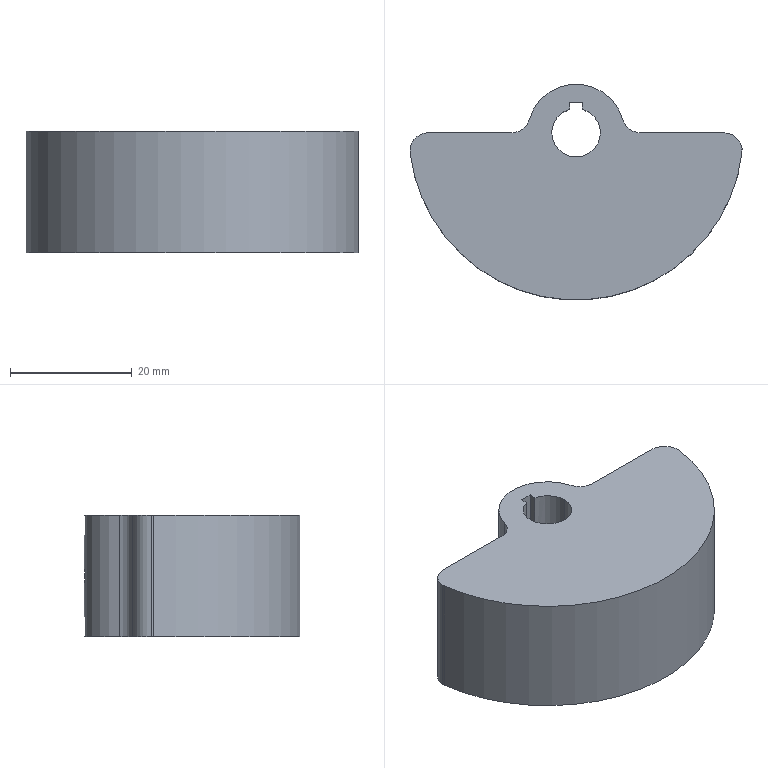Part | SolidWorks | features ICE 3, Extrusion 1, Fillet 1, HoleWzd 1 | 1 solid | 26 faces | box 54.631 x 35.5 x 20 mm | volume 24661 mm3 | cylinder 14 | plane 10 | cone 2 | commonest cylinder face diameters 6 x5 2.5 x4 8 x3 16 x1 55 x1
STEP:
#1=CARTESIAN_POINT('',(0.,-4.001,8.75));
#2=VERTEX_POINT('',#1);
#3=CARTESIAN_POINT('',(0.,-4.001,11.25));
#4=VERTEX_POINT('',#3);
#5=CARTESIAN_POINT('',(0.,-4.001,10.));
#6=DIRECTION('',(0.,1.,0.));
#7=DIRECTION('',(0.,0.,1.));
#8=AXIS2_PLACEMENT_3D('',#5,#6,#7);
#9=CIRCLE('',#8,1.25);
#10=EDGE_CURVE('',#2,#4,#9,.T.);
#11=ORIENTED_EDGE('',*,*,#10,.F.);
#12=CARTESIAN_POINT('',(0.,-4.,8.75));
#13=VERTEX_POINT('',#12);
#14=CARTESIAN_POINT('',(0.,8.,8.75));
#15=DIRECTION('',(0.,1.,0.));
#16=VECTOR('',#15,1000.);
#17=LINE('',#14,#16);
#18=EDGE_CURVE('',#2,#13,#17,.T.);
#19=ORIENTED_EDGE('',*,*,#18,.T.);
#20=CARTESIAN_POINT('',(0.,-4.,11.25));
#21=VERTEX_POINT('',#20);
#22=CARTESIAN_POINT('',(0.,-4.,11.25));
#23=CARTESIAN_POINT('',(-0.1663,-4.,11.25));
#24=CARTESIAN_POINT('',(-0.3294,-3.989,11.217));
#25=CARTESIAN_POINT('',(-0.6318,-3.953,11.091));
#26=CARTESIAN_POINT('',(-0.7697,-3.927,10.998));
#27=CARTESIAN_POINT('',(-0.9987,-3.875,10.769));
#28=CARTESIAN_POINT('',(-1.092,-3.849,10.63));
#29=CARTESIAN_POINT('',(-1.217,-3.811,10.33));
#30=CARTESIAN_POINT('',(-1.25,-3.8,10.165));
#31=CARTESIAN_POINT('',(-1.25,-3.8,9.918));
#32=CARTESIAN_POINT('',(-1.242,-3.802,9.835));
#33=CARTESIAN_POINT('',(-1.21,-3.813,9.674));
#34=CARTESIAN_POINT('',(-1.186,-3.82,9.596));
#35=CARTESIAN_POINT('',(-1.091,-3.849,9.368));
#36=CARTESIAN_POINT('',(-0.9989,-3.875,9.231));
#37=CARTESIAN_POINT('',(-0.8259,-3.914,9.058));
#38=CARTESIAN_POINT('',(-0.7634,-3.927,9.007));
#39=CARTESIAN_POINT('',(-0.6283,-3.951,8.916));
#40=CARTESIAN_POINT('',(-0.5551,-3.962,8.877));
#41=CARTESIAN_POINT('',(-0.3291,-3.989,8.783));
#42=CARTESIAN_POINT('',(-0.1639,-4.,8.75));
#43=CARTESIAN_POINT('',(0.,-4.,8.75));
#44=B_SPLINE_CURVE_WITH_KNOTS('',3,(#22,#23,#24,#25,#26,#27,#28,#29,#30,#31,#32,#33,#34,#35,#36,#37,#38,#39,#40,#41,#42,#43),.UNSPECIFIED.,.F.,.F.,(4,2,2,2,2,2,2,2,2,2,4),(0.,0.0004916,0.0009832,0.001475,0.001966,0.002212,0.002458,0.00295,0.003195,0.003441,0.003933),.UNSPECIFIED.);
#45=EDGE_CURVE('',#21,#13,#44,.T.);
#46=ORIENTED_EDGE('',*,*,#45,.F.);
#47=CARTESIAN_POINT('',(0.,8.,11.25));
#48=DIRECTION('',(0.,1.,0.));
#49=VECTOR('',#48,1000.);
#50=LINE('',#47,#49);
#51=EDGE_CURVE('',#4,#21,#50,.T.);
#52=ORIENTED_EDGE('',*,*,#51,.F.);
#53=EDGE_LOOP('',(#11,#19,#46,#52));
#54=FACE_OUTER_BOUND('',#53,.T.);
#55=CARTESIAN_POINT('',(0.,8.,10.));
#56=DIRECTION('',(0.,1.,0.));
#57=DIRECTION('',(0.,0.,1.));
#58=AXIS2_PLACEMENT_3D('',#55,#56,#57);
#59=CYLINDRICAL_SURFACE('',#58,1.25);
#60=ADVANCED_FACE('',(#54),#59,.F.);
#61=CARTESIAN_POINT('',(0.,-4.752,10.));
#62=VERTEX_POINT('',#61);
#63=CARTESIAN_POINT('',(0.,-4.001,11.25));
#64=DIRECTION('',(0.,0.515,0.8572));
#65=VECTOR('',#64,1000.);
#66=LINE('',#63,#65);
#67=EDGE_CURVE('',#62,#4,#66,.T.);
#68=ORIENTED_EDGE('',*,*,#67,.F.);
#69=CARTESIAN_POINT('',(0.,-4.001,8.75));
#70=DIRECTION('',(0.,0.515,-0.8572));
#71=VECTOR('',#70,1000.);
#72=LINE('',#69,#71);
#73=EDGE_CURVE('',#62,#2,#72,.T.);
#74=ORIENTED_EDGE('',*,*,#73,.T.);
#75=ORIENTED_EDGE('',*,*,#10,.T.);
#76=EDGE_LOOP('',(#68,#74,#75));
#77=FACE_OUTER_BOUND('',#76,.T.);
#78=CARTESIAN_POINT('',(0.,-4.001,10.));
#79=DIRECTION('',(0.,1.,0.));
#80=DIRECTION('',(0.,0.,1.));
#81=AXIS2_PLACEMENT_3D('',#78,#79,#80);
#82=CONICAL_SURFACE('',#81,1.25,1.03);
#83=ADVANCED_FACE('',(#77),#82,.F.);
#84=CARTESIAN_POINT('',(0.,5.,8.75));
#85=VERTEX_POINT('',#84);
#86=CARTESIAN_POINT('',(-1.,5.,9.25));
#87=VERTEX_POINT('',#86);
#88=CARTESIAN_POINT('',(0.,5.,10.));
#89=DIRECTION('',(0.,1.,0.));
#90=DIRECTION('',(0.,0.,1.));
#91=AXIS2_PLACEMENT_3D('',#88,#89,#90);
#92=CIRCLE('',#91,1.25);
#93=EDGE_CURVE('',#85,#87,#92,.T.);
#94=ORIENTED_EDGE('',*,*,#93,.F.);
#95=CARTESIAN_POINT('',(0.,8.,8.75));
#96=VERTEX_POINT('',#95);
#97=CARTESIAN_POINT('',(0.,8.,8.75));
#98=DIRECTION('',(0.,1.,0.));
#99=VECTOR('',#98,1000.);
#100=LINE('',#97,#99);
#101=EDGE_CURVE('',#85,#96,#100,.T.);
#102=ORIENTED_EDGE('',*,*,#101,.T.);
#103=CARTESIAN_POINT('',(0.,8.,11.25));
#104=VERTEX_POINT('',#103);
#105=CARTESIAN_POINT('',(0.,8.,8.75));
#106=CARTESIAN_POINT('',(-0.1633,8.,8.75));
#107=CARTESIAN_POINT('',(-0.3279,7.995,8.783));
#108=CARTESIAN_POINT('',(-0.6288,7.977,8.907));
#109=CARTESIAN_POINT('',(-0.768,7.964,9.));
#110=CARTESIAN_POINT('',(-0.941,7.945,9.173));
#111=CARTESIAN_POINT('',(-0.9937,7.938,9.237));
#112=CARTESIAN_POINT('',(-1.084,7.926,9.373));
#113=CARTESIAN_POINT('',(-1.123,7.921,9.445));
#114=CARTESIAN_POINT('',(-1.217,7.907,9.672));
#115=CARTESIAN_POINT('',(-1.25,7.902,9.834));
#116=CARTESIAN_POINT('',(-1.25,7.902,10.164));
#117=CARTESIAN_POINT('',(-1.218,7.907,10.327));
#118=CARTESIAN_POINT('',(-1.092,7.925,10.629));
#119=CARTESIAN_POINT('',(-0.9995,7.938,10.768));
#120=CARTESIAN_POINT('',(-0.7695,7.964,10.998));
#121=CARTESIAN_POINT('',(-0.6303,7.977,11.092));
#122=CARTESIAN_POINT('',(-0.3297,7.995,11.217));
#123=CARTESIAN_POINT('',(-0.1654,8.,11.25));
#124=CARTESIAN_POINT('',(0.,8.,11.25));
#125=B_SPLINE_CURVE_WITH_KNOTS('',3,(#105,#106,#107,#108,#109,#110,#111,#112,#113,#114,#115,#116,#117,#118,#119,#120,#121,#122,#123,#124),.UNSPECIFIED.,.F.,.F.,(4,2,2,2,2,2,2,2,2,4),(0.003914,0.004403,0.004892,0.005137,0.005381,0.005871,0.00636,0.006849,0.007338,0.007827),.UNSPECIFIED.);
#126=EDGE_CURVE('',#96,#104,#125,.T.);
#127=ORIENTED_EDGE('',*,*,#126,.T.);
#128=CARTESIAN_POINT('',(0.,5.,11.25));
#129=VERTEX_POINT('',#128);
#130=CARTESIAN_POINT('',(0.,8.,11.25));
#131=DIRECTION('',(0.,1.,0.));
#132=VECTOR('',#131,1000.);
#133=LINE('',#130,#132);
#134=EDGE_CURVE('',#129,#104,#133,.T.);
#135=ORIENTED_EDGE('',*,*,#134,.F.);
#136=CARTESIAN_POINT('',(-1.,5.,10.75));
#137=VERTEX_POINT('',#136);
#138=CARTESIAN_POINT('',(0.,5.,10.));
#139=DIRECTION('',(0.,1.,0.));
#140=DIRECTION('',(0.,0.,1.));
#141=AXIS2_PLACEMENT_3D('',#138,#139,#140);
#142=CIRCLE('',#141,1.25);
#143=EDGE_CURVE('',#137,#129,#142,.T.);
#144=ORIENTED_EDGE('',*,*,#143,.F.);
#145=CARTESIAN_POINT('',(-1.,3.873,10.75));
#146=VERTEX_POINT('',#145);
#147=CARTESIAN_POINT('',(-1.,8.,10.75));
#148=DIRECTION('',(0.,1.,0.));
#149=VECTOR('',#148,1000.);
#150=LINE('',#147,#149);
#151=EDGE_CURVE('',#146,#137,#150,.T.);
#152=ORIENTED_EDGE('',*,*,#151,.F.);
#153=CARTESIAN_POINT('',(-1.,3.873,9.25));
#154=VERTEX_POINT('',#153);
#155=CARTESIAN_POINT('',(-1.,3.873,9.25));
#156=CARTESIAN_POINT('',(-1.081,3.852,9.357));
#157=CARTESIAN_POINT('',(-1.142,3.834,9.475));
#158=CARTESIAN_POINT('',(-1.228,3.807,9.731));
#159=CARTESIAN_POINT('',(-1.25,3.8,9.864));
#160=CARTESIAN_POINT('',(-1.25,3.8,10.27));
#161=CARTESIAN_POINT('',(-1.161,3.831,10.535));
#162=CARTESIAN_POINT('',(-1.,3.873,10.75));
#163=B_SPLINE_CURVE_WITH_KNOTS('',3,(#155,#156,#157,#158,#159,#160,#161,#162),.UNSPECIFIED.,.F.,.F.,(4,2,2,4),(0.,0.0004023,0.0008046,0.001609),.UNSPECIFIED.);
#164=EDGE_CURVE('',#154,#146,#163,.T.);
#165=ORIENTED_EDGE('',*,*,#164,.F.);
#166=CARTESIAN_POINT('',(-1.,8.,9.25));
#167=DIRECTION('',(0.,-1.,0.));
#168=VECTOR('',#167,1000.);
#169=LINE('',#166,#168);
#170=EDGE_CURVE('',#87,#154,#169,.T.);
#171=ORIENTED_EDGE('',*,*,#170,.F.);
#172=EDGE_LOOP('',(#94,#102,#127,#135,#144,#152,#165,#171));
#173=FACE_OUTER_BOUND('',#172,.T.);
#174=CARTESIAN_POINT('',(0.,8.,10.));
#175=DIRECTION('',(0.,1.,0.));
#176=DIRECTION('',(0.,0.,1.));
#177=AXIS2_PLACEMENT_3D('',#174,#175,#176);
#178=CYLINDRICAL_SURFACE('',#177,1.25);
#179=ADVANCED_FACE('',(#173),#178,.F.);
#180=CARTESIAN_POINT('',(-27.316,-3.,20.));
#181=VERTEX_POINT('',#180);
#182=CARTESIAN_POINT('',(-27.293,-3.367,20.));
#183=VERTEX_POINT('',#182);
#184=CARTESIAN_POINT('',(-24.316,-3.,20.));
#185=DIRECTION('',(0.,0.,1.));
#186=DIRECTION('',(1.,0.,0.));
#187=AXIS2_PLACEMENT_3D('',#184,#185,#186);
#188=CIRCLE('',#187,3.);
#189=EDGE_CURVE('',#181,#183,#188,.T.);
#190=ORIENTED_EDGE('',*,*,#189,.F.);
#191=CARTESIAN_POINT('',(-27.316,-3.,0.));
#192=VERTEX_POINT('',#191);
#193=CARTESIAN_POINT('',(-27.316,-3.,20.));
#194=DIRECTION('',(0.,0.,-1.));
#195=VECTOR('',#194,1000.);
#196=LINE('',#193,#195);
#197=EDGE_CURVE('',#181,#192,#196,.T.);
#198=ORIENTED_EDGE('',*,*,#197,.T.);
#199=CARTESIAN_POINT('',(-27.293,-3.367,0.));
#200=VERTEX_POINT('',#199);
#201=CARTESIAN_POINT('',(-24.316,-3.,0.));
#202=DIRECTION('',(0.,0.,-1.));
#203=DIRECTION('',(1.,0.,0.));
#204=AXIS2_PLACEMENT_3D('',#201,#202,#203);
#205=CIRCLE('',#204,3.);
#206=EDGE_CURVE('',#200,#192,#205,.T.);
#207=ORIENTED_EDGE('',*,*,#206,.F.);
#208=CARTESIAN_POINT('',(-27.293,-3.367,20.));
#209=DIRECTION('',(0.,0.,-1.));
#210=VECTOR('',#209,1000.);
#211=LINE('',#208,#210);
#212=EDGE_CURVE('',#183,#200,#211,.T.);
#213=ORIENTED_EDGE('',*,*,#212,.F.);
#214=EDGE_LOOP('',(#190,#198,#207,#213));
#215=FACE_OUTER_BOUND('',#214,.T.);
#216=CARTESIAN_POINT('',(-24.316,-3.,20.));
#217=DIRECTION('',(0.,0.,-1.));
#218=DIRECTION('',(-1.,0.,0.));
#219=AXIS2_PLACEMENT_3D('',#216,#217,#218);
#220=CYLINDRICAL_SURFACE('',#219,3.);
#221=ADVANCED_FACE('',(#215),#220,.T.);
#222=ORIENTED_EDGE('',*,*,#45,.T.);
#223=CARTESIAN_POINT('',(0.,-4.,8.75));
#224=CARTESIAN_POINT('',(0.1638,-4.,8.75));
#225=CARTESIAN_POINT('',(0.3292,-3.989,8.783));
#226=CARTESIAN_POINT('',(0.6307,-3.953,8.908));
#227=CARTESIAN_POINT('',(0.7685,-3.927,9.001));
#228=CARTESIAN_POINT('',(0.9992,-3.875,9.231));
#229=CARTESIAN_POINT('',(1.091,-3.849,9.368));
#230=CARTESIAN_POINT('',(1.186,-3.82,9.596));
#231=CARTESIAN_POINT('',(1.21,-3.813,9.674));
#232=CARTESIAN_POINT('',(1.242,-3.802,9.834));
#233=CARTESIAN_POINT('',(1.25,-3.8,9.918));
#234=CARTESIAN_POINT('',(1.25,-3.8,10.165));
#235=CARTESIAN_POINT('',(1.217,-3.811,10.329));
#236=CARTESIAN_POINT('',(1.092,-3.849,10.631));
#237=CARTESIAN_POINT('',(0.9987,-3.875,10.769));
#238=CARTESIAN_POINT('',(0.7696,-3.927,10.998));
#239=CARTESIAN_POINT('',(0.6317,-3.953,11.091));
#240=CARTESIAN_POINT('',(0.3299,-3.989,11.217));
#241=CARTESIAN_POINT('',(0.1663,-4.,11.25));
#242=CARTESIAN_POINT('',(0.,-4.,11.25));
#243=B_SPLINE_CURVE_WITH_KNOTS('',3,(#223,#224,#225,#226,#227,#228,#229,#230,#231,#232,#233,#234,#235,#236,#237,#238,#239,#240,#241,#242),.UNSPECIFIED.,.F.,.F.,(4,2,2,2,2,2,2,2,2,4),(0.003933,0.004424,0.004916,0.005407,0.005653,0.005899,0.00639,0.006882,0.007373,0.007865),.UNSPECIFIED.);
#244=EDGE_CURVE('',#13,#21,#243,.T.);
#245=ORIENTED_EDGE('',*,*,#244,.T.);
#246=EDGE_LOOP('',(#222,#245));
#247=FACE_BOUND('',#246,.T.);
#248=CARTESIAN_POINT('',(-4.,0.,0.));
#249=VERTEX_POINT('',#248);
#250=CARTESIAN_POINT('',(4.,0.,0.));
#251=VERTEX_POINT('',#250);
#252=CARTESIAN_POINT('',(0.,0.,0.));
#253=DIRECTION('',(0.,0.,1.));
#254=DIRECTION('',(1.,0.,0.));
#255=AXIS2_PLACEMENT_3D('',#252,#253,#254);
#256=CIRCLE('',#255,4.);
#257=EDGE_CURVE('',#249,#251,#256,.T.);
#258=ORIENTED_EDGE('',*,*,#257,.F.);
#259=CARTESIAN_POINT('',(-4.,0.,20.));
#260=VERTEX_POINT('',#259);
#261=CARTESIAN_POINT('',(-4.,0.,0.));
#262=DIRECTION('',(0.,0.,1.));
#263=VECTOR('',#262,1000.);
#264=LINE('',#261,#263);
#265=EDGE_CURVE('',#249,#260,#264,.T.);
#266=ORIENTED_EDGE('',*,*,#265,.T.);
#267=CARTESIAN_POINT('',(4.,0.,20.));
#268=VERTEX_POINT('',#267);
#269=CARTESIAN_POINT('',(0.,0.,20.));
#270=DIRECTION('',(0.,0.,1.));
#271=DIRECTION('',(1.,0.,0.));
#272=AXIS2_PLACEMENT_3D('',#269,#270,#271);
#273=CIRCLE('',#272,4.);
#274=EDGE_CURVE('',#260,#268,#273,.T.);
#275=ORIENTED_EDGE('',*,*,#274,.T.);
#276=CARTESIAN_POINT('',(4.,0.,0.));
#277=DIRECTION('',(0.,0.,1.));
#278=VECTOR('',#277,1000.);
#279=LINE('',#276,#278);
#280=EDGE_CURVE('',#251,#268,#279,.T.);
#281=ORIENTED_EDGE('',*,*,#280,.F.);
#282=EDGE_LOOP('',(#258,#266,#275,#281));
#283=FACE_OUTER_BOUND('',#282,.T.);
#284=CARTESIAN_POINT('',(0.,0.,0.));
#285=DIRECTION('',(0.,0.,1.));
#286=DIRECTION('',(1.,0.,0.));
#287=AXIS2_PLACEMENT_3D('',#284,#285,#286);
#288=CYLINDRICAL_SURFACE('',#287,4.);
#289=ADVANCED_FACE('',(#247,#283),#288,.F.);
#290=CARTESIAN_POINT('',(1.,3.873,0.));
#291=VERTEX_POINT('',#290);
#292=CARTESIAN_POINT('',(0.,0.,0.));
#293=DIRECTION('',(0.,0.,1.));
#294=DIRECTION('',(1.,0.,0.));
#295=AXIS2_PLACEMENT_3D('',#292,#293,#294);
#296=CIRCLE('',#295,4.);
#297=EDGE_CURVE('',#251,#291,#296,.T.);
#298=ORIENTED_EDGE('',*,*,#297,.F.);
#299=ORIENTED_EDGE('',*,*,#280,.T.);
#300=CARTESIAN_POINT('',(1.,3.873,20.));
#301=VERTEX_POINT('',#300);
#302=CARTESIAN_POINT('',(0.,0.,20.));
#303=DIRECTION('',(0.,0.,1.));
#304=DIRECTION('',(1.,0.,0.));
#305=AXIS2_PLACEMENT_3D('',#302,#303,#304);
#306=CIRCLE('',#305,4.);
#307=EDGE_CURVE('',#268,#301,#306,.T.);
#308=ORIENTED_EDGE('',*,*,#307,.T.);
#309=CARTESIAN_POINT('',(1.,3.873,10.75));
#310=VERTEX_POINT('',#309);
#311=CARTESIAN_POINT('',(1.,3.873,0.));
#312=DIRECTION('',(0.,0.,-1.));
#313=VECTOR('',#312,1000.);
#314=LINE('',#311,#313);
#315=EDGE_CURVE('',#301,#310,#314,.T.);
#316=ORIENTED_EDGE('',*,*,#315,.T.);
#317=CARTESIAN_POINT('',(1.,3.873,9.25));
#318=VERTEX_POINT('',#317);
#319=CARTESIAN_POINT('',(1.,3.873,10.75));
#320=CARTESIAN_POINT('',(1.081,3.852,10.643));
#321=CARTESIAN_POINT('',(1.142,3.834,10.525));
#322=CARTESIAN_POINT('',(1.228,3.807,10.269));
#323=CARTESIAN_POINT('',(1.25,3.8,10.136));
#324=CARTESIAN_POINT('',(1.25,3.8,9.73));
#325=CARTESIAN_POINT('',(1.161,3.831,9.465));
#326=CARTESIAN_POINT('',(1.,3.873,9.25));
#327=B_SPLINE_CURVE_WITH_KNOTS('',3,(#319,#320,#321,#322,#323,#324,#325,#326),.UNSPECIFIED.,.F.,.F.,(4,2,2,4),(0.,0.0004023,0.0008046,0.001609),.UNSPECIFIED.);
#328=EDGE_CURVE('',#310,#318,#327,.T.);
#329=ORIENTED_EDGE('',*,*,#328,.T.);
#330=CARTESIAN_POINT('',(1.,3.873,0.));
#331=DIRECTION('',(0.,0.,-1.));
#332=VECTOR('',#331,1000.);
#333=LINE('',#330,#332);
#334=EDGE_CURVE('',#318,#291,#333,.T.);
#335=ORIENTED_EDGE('',*,*,#334,.T.);
#336=EDGE_LOOP('',(#298,#299,#308,#316,#329,#335));
#337=FACE_OUTER_BOUND('',#336,.T.);
#338=CARTESIAN_POINT('',(0.,0.,0.));
#339=DIRECTION('',(0.,0.,1.));
#340=DIRECTION('',(1.,0.,0.));
#341=AXIS2_PLACEMENT_3D('',#338,#339,#340);
#342=CYLINDRICAL_SURFACE('',#341,4.);
#343=ADVANCED_FACE('',(#337),#342,.F.);
#344=CARTESIAN_POINT('',(-1.,3.873,20.));
#345=VERTEX_POINT('',#344);
#346=CARTESIAN_POINT('',(-1.,3.873,0.));
#347=DIRECTION('',(0.,0.,1.));
#348=VECTOR('',#347,1000.);
#349=LINE('',#346,#348);
#350=EDGE_CURVE('',#146,#345,#349,.T.);
#351=ORIENTED_EDGE('',*,*,#350,.F.);
#352=ORIENTED_EDGE('',*,*,#151,.T.);
#353=CARTESIAN_POINT('',(-1.,5.,20.));
#354=VERTEX_POINT('',#353);
#355=CARTESIAN_POINT('',(-1.,5.,0.));
#356=DIRECTION('',(0.,0.,1.));
#357=VECTOR('',#356,1000.);
#358=LINE('',#355,#357);
#359=EDGE_CURVE('',#137,#354,#358,.T.);
#360=ORIENTED_EDGE('',*,*,#359,.T.);
#361=CARTESIAN_POINT('',(-1.,3.,20.));
#362=DIRECTION('',(0.,-1.,0.));
#363=VECTOR('',#362,1000.);
#364=LINE('',#361,#363);
#365=EDGE_CURVE('',#354,#345,#364,.T.);
#366=ORIENTED_EDGE('',*,*,#365,.T.);
#367=EDGE_LOOP('',(#351,#352,#360,#366));
#368=FACE_OUTER_BOUND('',#367,.T.);
#369=CARTESIAN_POINT('',(-1.,3.,0.));
#370=DIRECTION('',(-1.,0.,0.));
#371=DIRECTION('',(0.,0.,1.));
#372=AXIS2_PLACEMENT_3D('',#369,#370,#371);
#373=PLANE('',#372);
#374=ADVANCED_FACE('',(#368),#373,.F.);
#375=CARTESIAN_POINT('',(1.,5.,0.));
#376=VERTEX_POINT('',#375);
#377=CARTESIAN_POINT('',(1.,5.,9.25));
#378=VERTEX_POINT('',#377);
#379=CARTESIAN_POINT('',(1.,5.,0.));
#380=DIRECTION('',(0.,0.,1.));
#381=VECTOR('',#380,1000.);
#382=LINE('',#379,#381);
#383=EDGE_CURVE('',#376,#378,#382,.T.);
#384=ORIENTED_EDGE('',*,*,#383,.T.);
#385=CARTESIAN_POINT('',(0.,5.,10.));
#386=DIRECTION('',(0.,1.,0.));
#387=DIRECTION('',(0.,0.,1.));
#388=AXIS2_PLACEMENT_3D('',#385,#386,#387);
#389=CIRCLE('',#388,1.25);
#390=EDGE_CURVE('',#378,#85,#389,.T.);
#391=ORIENTED_EDGE('',*,*,#390,.T.);
#392=ORIENTED_EDGE('',*,*,#93,.T.);
#393=CARTESIAN_POINT('',(-1.,5.,0.));
#394=VERTEX_POINT('',#393);
#395=CARTESIAN_POINT('',(-1.,5.,0.));
#396=DIRECTION('',(0.,0.,1.));
#397=VECTOR('',#396,1000.);
#398=LINE('',#395,#397);
#399=EDGE_CURVE('',#394,#87,#398,.T.);
#400=ORIENTED_EDGE('',*,*,#399,.F.);
#401=CARTESIAN_POINT('',(-1.,5.,0.));
#402=DIRECTION('',(-1.,0.,0.));
#403=VECTOR('',#402,1000.);
#404=LINE('',#401,#403);
#405=EDGE_CURVE('',#376,#394,#404,.T.);
#406=ORIENTED_EDGE('',*,*,#405,.F.);
#407=EDGE_LOOP('',(#384,#391,#392,#400,#406));
#408=FACE_OUTER_BOUND('',#407,.T.);
#409=CARTESIAN_POINT('',(-1.,5.,0.));
#410=DIRECTION('',(0.,1.,0.));
#411=DIRECTION('',(0.,0.,1.));
#412=AXIS2_PLACEMENT_3D('',#409,#410,#411);
#413=PLANE('',#412);
#414=ADVANCED_FACE('',(#408),#413,.F.);
#415=ORIENTED_EDGE('',*,*,#334,.F.);
#416=CARTESIAN_POINT('',(1.,8.,9.25));
#417=DIRECTION('',(0.,1.,0.));
#418=VECTOR('',#417,1000.);
#419=LINE('',#416,#418);
#420=EDGE_CURVE('',#318,#378,#419,.T.);
#421=ORIENTED_EDGE('',*,*,#420,.T.);
#422=ORIENTED_EDGE('',*,*,#383,.F.);
#423=CARTESIAN_POINT('',(1.,3.,0.));
#424=DIRECTION('',(0.,1.,0.));
#425=VECTOR('',#424,1000.);
#426=LINE('',#423,#425);
#427=EDGE_CURVE('',#291,#376,#426,.T.);
#428=ORIENTED_EDGE('',*,*,#427,.F.);
#429=EDGE_LOOP('',(#415,#421,#422,#428));
#430=FACE_OUTER_BOUND('',#429,.T.);
#431=CARTESIAN_POINT('',(1.,3.,0.));
#432=DIRECTION('',(1.,0.,0.));
#433=DIRECTION('',(0.,0.,-1.));
#434=AXIS2_PLACEMENT_3D('',#431,#432,#433);
#435=PLANE('',#434);
#436=ADVANCED_FACE('',(#430),#435,.F.);
#437=CARTESIAN_POINT('',(24.316,0.,20.));
#438=VERTEX_POINT('',#437);
#439=CARTESIAN_POINT('',(10.583,0.,20.));
#440=VERTEX_POINT('',#439);
#441=CARTESIAN_POINT('',(-27.5,0.,20.));
#442=DIRECTION('',(-1.,0.,0.));
#443=VECTOR('',#442,1000.);
#444=LINE('',#441,#443);
#445=EDGE_CURVE('',#438,#440,#444,.T.);
#446=ORIENTED_EDGE('',*,*,#445,.F.);
#447=CARTESIAN_POINT('',(24.316,0.,0.));
#448=VERTEX_POINT('',#447);
#449=CARTESIAN_POINT('',(24.316,0.,20.));
#450=DIRECTION('',(0.,0.,-1.));
#451=VECTOR('',#450,1000.);
#452=LINE('',#449,#451);
#453=EDGE_CURVE('',#438,#448,#452,.T.);
#454=ORIENTED_EDGE('',*,*,#453,.T.);
#455=CARTESIAN_POINT('',(10.583,0.,0.));
#456=VERTEX_POINT('',#455);
#457=CARTESIAN_POINT('',(-27.5,0.,0.));
#458=DIRECTION('',(-1.,0.,0.));
#459=VECTOR('',#458,1000.);
#460=LINE('',#457,#459);
#461=EDGE_CURVE('',#448,#456,#460,.T.);
#462=ORIENTED_EDGE('',*,*,#461,.T.);
#463=CARTESIAN_POINT('',(10.583,0.,20.));
#464=DIRECTION('',(0.,0.,1.));
#465=VECTOR('',#464,1000.);
#466=LINE('',#463,#465);
#467=EDGE_CURVE('',#456,#440,#466,.T.);
#468=ORIENTED_EDGE('',*,*,#467,.T.);
#469=EDGE_LOOP('',(#446,#454,#462,#468));
#470=FACE_OUTER_BOUND('',#469,.T.);
#471=CARTESIAN_POINT('',(-27.5,0.,20.));
#472=DIRECTION('',(0.,-1.,0.));
#473=DIRECTION('',(0.,0.,-1.));
#474=AXIS2_PLACEMENT_3D('',#471,#472,#473);
#475=PLANE('',#474);
#476=ADVANCED_FACE('',(#470),#475,.F.);
#477=CARTESIAN_POINT('',(27.293,-3.367,0.));
#478=VERTEX_POINT('',#477);
#479=CARTESIAN_POINT('',(0.,0.,0.));
#480=DIRECTION('',(0.,0.,1.));
#481=DIRECTION('',(1.,0.,0.));
#482=AXIS2_PLACEMENT_3D('',#479,#480,#481);
#483=CIRCLE('',#482,27.5);
#484=EDGE_CURVE('',#200,#478,#483,.T.);
#485=ORIENTED_EDGE('',*,*,#484,.T.);
#486=CARTESIAN_POINT('',(27.293,-3.367,20.));
#487=VERTEX_POINT('',#486);
#488=CARTESIAN_POINT('',(27.293,-3.367,20.));
#489=DIRECTION('',(0.,0.,1.));
#490=VECTOR('',#489,1000.);
#491=LINE('',#488,#490);
#492=EDGE_CURVE('',#478,#487,#491,.T.);
#493=ORIENTED_EDGE('',*,*,#492,.T.);
#494=CARTESIAN_POINT('',(0.,0.,20.));
#495=DIRECTION('',(0.,0.,1.));
#496=DIRECTION('',(1.,0.,0.));
#497=AXIS2_PLACEMENT_3D('',#494,#495,#496);
#498=CIRCLE('',#497,27.5);
#499=EDGE_CURVE('',#183,#487,#498,.T.);
#500=ORIENTED_EDGE('',*,*,#499,.F.);
#501=ORIENTED_EDGE('',*,*,#212,.T.);
#502=EDGE_LOOP('',(#485,#493,#500,#501));
#503=FACE_OUTER_BOUND('',#502,.T.);
#504=CARTESIAN_POINT('',(0.,0.,20.));
#505=DIRECTION('',(0.,0.,-1.));
#506=DIRECTION('',(-1.,0.,0.));
#507=AXIS2_PLACEMENT_3D('',#504,#505,#506);
#508=CYLINDRICAL_SURFACE('',#507,27.5);
#509=ADVANCED_FACE('',(#503),#508,.T.);
#510=CARTESIAN_POINT('',(-10.583,0.,20.));
#511=VERTEX_POINT('',#510);
#512=CARTESIAN_POINT('',(-24.316,0.,20.));
#513=VERTEX_POINT('',#512);
#514=CARTESIAN_POINT('',(-27.5,0.,20.));
#515=DIRECTION('',(-1.,0.,0.));
#516=VECTOR('',#515,1000.);
#517=LINE('',#514,#516);
#518=EDGE_CURVE('',#511,#513,#517,.T.);
#519=ORIENTED_EDGE('',*,*,#518,.F.);
#520=CARTESIAN_POINT('',(-10.583,0.,0.));
#521=VERTEX_POINT('',#520);
#522=CARTESIAN_POINT('',(-10.583,0.,20.));
#523=DIRECTION('',(0.,0.,-1.));
#524=VECTOR('',#523,1000.);
#525=LINE('',#522,#524);
#526=EDGE_CURVE('',#511,#521,#525,.T.);
#527=ORIENTED_EDGE('',*,*,#526,.T.);
#528=CARTESIAN_POINT('',(-24.316,0.,0.));
#529=VERTEX_POINT('',#528);
#530=CARTESIAN_POINT('',(-27.5,0.,0.));
#531=DIRECTION('',(-1.,0.,0.));
#532=VECTOR('',#531,1000.);
#533=LINE('',#530,#532);
#534=EDGE_CURVE('',#521,#529,#533,.T.);
#535=ORIENTED_EDGE('',*,*,#534,.T.);
#536=CARTESIAN_POINT('',(-24.316,0.,20.));
#537=DIRECTION('',(0.,0.,1.));
#538=VECTOR('',#537,1000.);
#539=LINE('',#536,#538);
#540=EDGE_CURVE('',#529,#513,#539,.T.);
#541=ORIENTED_EDGE('',*,*,#540,.T.);
#542=EDGE_LOOP('',(#519,#527,#535,#541));
#543=FACE_OUTER_BOUND('',#542,.T.);
#544=CARTESIAN_POINT('',(-27.5,0.,20.));
#545=DIRECTION('',(0.,-1.,0.));
#546=DIRECTION('',(0.,0.,-1.));
#547=AXIS2_PLACEMENT_3D('',#544,#545,#546);
#548=PLANE('',#547);
#549=ADVANCED_FACE('',(#543),#548,.F.);
#550=CARTESIAN_POINT('',(1.,5.,20.));
#551=VERTEX_POINT('',#550);
#552=CARTESIAN_POINT('',(1.,3.,20.));
#553=DIRECTION('',(0.,1.,0.));
#554=VECTOR('',#553,1000.);
#555=LINE('',#552,#554);
#556=EDGE_CURVE('',#301,#551,#555,.T.);
#557=ORIENTED_EDGE('',*,*,#556,.F.);
#558=ORIENTED_EDGE('',*,*,#307,.F.);
#559=ORIENTED_EDGE('',*,*,#274,.F.);
#560=CARTESIAN_POINT('',(0.,0.,20.));
#561=DIRECTION('',(0.,0.,1.));
#562=DIRECTION('',(1.,0.,0.));
#563=AXIS2_PLACEMENT_3D('',#560,#561,#562);
#564=CIRCLE('',#563,4.);
#565=EDGE_CURVE('',#345,#260,#564,.T.);
#566=ORIENTED_EDGE('',*,*,#565,.F.);
#567=ORIENTED_EDGE('',*,*,#365,.F.);
#568=CARTESIAN_POINT('',(-1.,5.,20.));
#569=DIRECTION('',(-1.,0.,0.));
#570=VECTOR('',#569,1000.);
#571=LINE('',#568,#570);
#572=EDGE_CURVE('',#551,#354,#571,.T.);
#573=ORIENTED_EDGE('',*,*,#572,.F.);
#574=EDGE_LOOP('',(#557,#558,#559,#566,#567,#573));
#575=FACE_BOUND('',#574,.T.);
#576=ORIENTED_EDGE('',*,*,#499,.T.);
#577=CARTESIAN_POINT('',(24.316,-3.,20.));
#578=DIRECTION('',(0.,0.,1.));
#579=DIRECTION('',(1.,0.,0.));
#580=AXIS2_PLACEMENT_3D('',#577,#578,#579);
#581=CIRCLE('',#580,3.);
#582=EDGE_CURVE('',#487,#438,#581,.T.);
#583=ORIENTED_EDGE('',*,*,#582,.T.);
#584=ORIENTED_EDGE('',*,*,#445,.T.);
#585=CARTESIAN_POINT('',(7.697,2.182,20.));
#586=VERTEX_POINT('',#585);
#587=CARTESIAN_POINT('',(10.583,3.,20.));
#588=DIRECTION('',(0.,0.,-1.));
#589=DIRECTION('',(1.,0.,0.));
#590=AXIS2_PLACEMENT_3D('',#587,#588,#589);
#591=CIRCLE('',#590,3.);
#592=EDGE_CURVE('',#440,#586,#591,.T.);
#593=ORIENTED_EDGE('',*,*,#592,.T.);
#594=CARTESIAN_POINT('',(-7.697,2.182,20.));
#595=VERTEX_POINT('',#594);
#596=CARTESIAN_POINT('',(0.,0.,20.));
#597=DIRECTION('',(0.,0.,1.));
#598=DIRECTION('',(1.,0.,0.));
#599=AXIS2_PLACEMENT_3D('',#596,#597,#598);
#600=CIRCLE('',#599,8.);
#601=EDGE_CURVE('',#586,#595,#600,.T.);
#602=ORIENTED_EDGE('',*,*,#601,.T.);
#603=CARTESIAN_POINT('',(-10.583,3.,20.));
#604=DIRECTION('',(0.,0.,-1.));
#605=DIRECTION('',(1.,0.,0.));
#606=AXIS2_PLACEMENT_3D('',#603,#604,#605);
#607=CIRCLE('',#606,3.);
#608=EDGE_CURVE('',#595,#511,#607,.T.);
#609=ORIENTED_EDGE('',*,*,#608,.T.);
#610=ORIENTED_EDGE('',*,*,#518,.T.);
#611=CARTESIAN_POINT('',(-24.316,-3.,20.));
#612=DIRECTION('',(0.,0.,1.));
#613=DIRECTION('',(1.,0.,0.));
#614=AXIS2_PLACEMENT_3D('',#611,#612,#613);
#615=CIRCLE('',#614,3.);
#616=EDGE_CURVE('',#513,#181,#615,.T.);
#617=ORIENTED_EDGE('',*,*,#616,.T.);
#618=ORIENTED_EDGE('',*,*,#189,.T.);
#619=EDGE_LOOP('',(#576,#583,#584,#593,#602,#609,#610,#617,#618));
#620=FACE_OUTER_BOUND('',#619,.T.);
#621=CARTESIAN_POINT('',(0.,0.,20.));
#622=DIRECTION('',(0.,0.,1.));
#623=DIRECTION('',(1.,0.,0.));
#624=AXIS2_PLACEMENT_3D('',#621,#622,#623);
#625=PLANE('',#624);
#626=ADVANCED_FACE('',(#575,#620),#625,.T.);
#627=CARTESIAN_POINT('',(-1.,3.873,0.));
#628=VERTEX_POINT('',#627);
#629=CARTESIAN_POINT('',(0.,0.,0.));
#630=DIRECTION('',(0.,0.,1.));
#631=DIRECTION('',(1.,0.,0.));
#632=AXIS2_PLACEMENT_3D('',#629,#630,#631);
#633=CIRCLE('',#632,4.);
#634=EDGE_CURVE('',#628,#249,#633,.T.);
#635=ORIENTED_EDGE('',*,*,#634,.T.);
#636=ORIENTED_EDGE('',*,*,#257,.T.);
#637=ORIENTED_EDGE('',*,*,#297,.T.);
#638=ORIENTED_EDGE('',*,*,#427,.T.);
#639=ORIENTED_EDGE('',*,*,#405,.T.);
#640=CARTESIAN_POINT('',(-1.,3.,0.));
#641=DIRECTION('',(0.,-1.,0.));
#642=VECTOR('',#641,1000.);
#643=LINE('',#640,#642);
#644=EDGE_CURVE('',#394,#628,#643,.T.);
#645=ORIENTED_EDGE('',*,*,#644,.T.);
#646=EDGE_LOOP('',(#635,#636,#637,#638,#639,#645));
#647=FACE_BOUND('',#646,.T.);
#648=ORIENTED_EDGE('',*,*,#461,.F.);
#649=CARTESIAN_POINT('',(24.316,-3.,0.));
#650=DIRECTION('',(0.,0.,-1.));
#651=DIRECTION('',(1.,0.,0.));
#652=AXIS2_PLACEMENT_3D('',#649,#650,#651);
#653=CIRCLE('',#652,3.);
#654=EDGE_CURVE('',#448,#478,#653,.T.);
#655=ORIENTED_EDGE('',*,*,#654,.T.);
#656=ORIENTED_EDGE('',*,*,#484,.F.);
#657=ORIENTED_EDGE('',*,*,#206,.T.);
#658=CARTESIAN_POINT('',(-24.316,-3.,0.));
#659=DIRECTION('',(0.,0.,-1.));
#660=DIRECTION('',(1.,0.,0.));
#661=AXIS2_PLACEMENT_3D('',#658,#659,#660);
#662=CIRCLE('',#661,3.);
#663=EDGE_CURVE('',#192,#529,#662,.T.);
#664=ORIENTED_EDGE('',*,*,#663,.T.);
#665=ORIENTED_EDGE('',*,*,#534,.F.);
#666=CARTESIAN_POINT('',(-7.697,2.182,0.));
#667=VERTEX_POINT('',#666);
#668=CARTESIAN_POINT('',(-10.583,3.,0.));
#669=DIRECTION('',(0.,0.,1.));
#670=DIRECTION('',(1.,0.,0.));
#671=AXIS2_PLACEMENT_3D('',#668,#669,#670);
#672=CIRCLE('',#671,3.);
#673=EDGE_CURVE('',#521,#667,#672,.T.);
#674=ORIENTED_EDGE('',*,*,#673,.T.);
#675=CARTESIAN_POINT('',(7.697,2.182,0.));
#676=VERTEX_POINT('',#675);
#677=CARTESIAN_POINT('',(0.,0.,0.));
#678=DIRECTION('',(0.,0.,1.));
#679=DIRECTION('',(1.,0.,0.));
#680=AXIS2_PLACEMENT_3D('',#677,#678,#679);
#681=CIRCLE('',#680,8.);
#682=EDGE_CURVE('',#676,#667,#681,.T.);
#683=ORIENTED_EDGE('',*,*,#682,.F.);
#684=CARTESIAN_POINT('',(10.583,3.,0.));
#685=DIRECTION('',(0.,0.,1.));
#686=DIRECTION('',(1.,0.,0.));
#687=AXIS2_PLACEMENT_3D('',#684,#685,#686);
#688=CIRCLE('',#687,3.);
#689=EDGE_CURVE('',#676,#456,#688,.T.);
#690=ORIENTED_EDGE('',*,*,#689,.T.);
#691=EDGE_LOOP('',(#648,#655,#656,#657,#664,#665,#674,#683,#690));
#692=FACE_OUTER_BOUND('',#691,.T.);
#693=CARTESIAN_POINT('',(0.,0.,0.));
#694=DIRECTION('',(0.,0.,1.));
#695=DIRECTION('',(1.,0.,0.));
#696=AXIS2_PLACEMENT_3D('',#693,#694,#695);
#697=PLANE('',#696);
#698=ADVANCED_FACE('',(#647,#692),#697,.F.);
#699=CARTESIAN_POINT('',(0.,8.,11.25));
#700=CARTESIAN_POINT('',(0.1655,8.,11.25));
#701=CARTESIAN_POINT('',(0.3278,7.995,11.217));
#702=CARTESIAN_POINT('',(0.6305,7.977,11.092));
#703=CARTESIAN_POINT('',(0.769,7.964,10.999));
#704=CARTESIAN_POINT('',(0.9992,7.938,10.769));
#705=CARTESIAN_POINT('',(1.092,7.925,10.629));
#706=CARTESIAN_POINT('',(1.217,7.907,10.328));
#707=CARTESIAN_POINT('',(1.25,7.902,10.164));
#708=CARTESIAN_POINT('',(1.25,7.902,9.919));
#709=CARTESIAN_POINT('',(1.242,7.903,9.836));
#710=CARTESIAN_POINT('',(1.21,7.908,9.675));
#711=CARTESIAN_POINT('',(1.186,7.912,9.597));
#712=CARTESIAN_POINT('',(1.092,7.925,9.37));
#713=CARTESIAN_POINT('',(1.,7.938,9.233));
#714=CARTESIAN_POINT('',(0.7675,7.964,9.));
#715=CARTESIAN_POINT('',(0.6299,7.977,8.908));
#716=CARTESIAN_POINT('',(0.403,7.99,8.814));
#717=CARTESIAN_POINT('',(0.3251,7.994,8.79));
#718=CARTESIAN_POINT('',(0.1646,7.999,8.758));
#719=CARTESIAN_POINT('',(0.08165,8.,8.75));
#720=CARTESIAN_POINT('',(0.,8.,8.75));
#721=B_SPLINE_CURVE_WITH_KNOTS('',3,(#699,#700,#701,#702,#703,#704,#705,#706,#707,#708,#709,#710,#711,#712,#713,#714,#715,#716,#717,#718,#719,#720),.UNSPECIFIED.,.F.,.F.,(4,2,2,2,2,2,2,2,2,2,4),(0.,0.0004893,0.0009785,0.001468,0.001957,0.002202,0.002446,0.002936,0.003425,0.003669,0.003914),.UNSPECIFIED.);
#722=EDGE_CURVE('',#104,#96,#721,.T.);
#723=ORIENTED_EDGE('',*,*,#722,.F.);
#724=ORIENTED_EDGE('',*,*,#126,.F.);
#725=EDGE_LOOP('',(#723,#724));
#726=FACE_BOUND('',#725,.T.);
#727=ORIENTED_EDGE('',*,*,#601,.F.);
#728=CARTESIAN_POINT('',(7.697,2.182,0.));
#729=DIRECTION('',(0.,0.,-1.));
#730=VECTOR('',#729,1000.);
#731=LINE('',#728,#730);
#732=EDGE_CURVE('',#586,#676,#731,.T.);
#733=ORIENTED_EDGE('',*,*,#732,.T.);
#734=ORIENTED_EDGE('',*,*,#682,.T.);
#735=CARTESIAN_POINT('',(-7.697,2.182,0.));
#736=DIRECTION('',(0.,0.,1.));
#737=VECTOR('',#736,1000.);
#738=LINE('',#735,#737);
#739=EDGE_CURVE('',#667,#595,#738,.T.);
#740=ORIENTED_EDGE('',*,*,#739,.T.);
#741=EDGE_LOOP('',(#727,#733,#734,#740));
#742=FACE_OUTER_BOUND('',#741,.T.);
#743=CARTESIAN_POINT('',(0.,0.,0.));
#744=DIRECTION('',(0.,0.,1.));
#745=DIRECTION('',(1.,0.,0.));
#746=AXIS2_PLACEMENT_3D('',#743,#744,#745);
#747=CYLINDRICAL_SURFACE('',#746,8.);
#748=ADVANCED_FACE('',(#726,#742),#747,.T.);
#749=ORIENTED_EDGE('',*,*,#265,.F.);
#750=ORIENTED_EDGE('',*,*,#634,.F.);
#751=CARTESIAN_POINT('',(-1.,3.873,0.));
#752=DIRECTION('',(0.,0.,1.));
#753=VECTOR('',#752,1000.);
#754=LINE('',#751,#753);
#755=EDGE_CURVE('',#628,#154,#754,.T.);
#756=ORIENTED_EDGE('',*,*,#755,.T.);
#757=ORIENTED_EDGE('',*,*,#164,.T.);
#758=ORIENTED_EDGE('',*,*,#350,.T.);
#759=ORIENTED_EDGE('',*,*,#565,.T.);
#760=EDGE_LOOP('',(#749,#750,#756,#757,#758,#759));
#761=FACE_OUTER_BOUND('',#760,.T.);
#762=CARTESIAN_POINT('',(0.,0.,0.));
#763=DIRECTION('',(0.,0.,1.));
#764=DIRECTION('',(1.,0.,0.));
#765=AXIS2_PLACEMENT_3D('',#762,#763,#764);
#766=CYLINDRICAL_SURFACE('',#765,4.);
#767=ADVANCED_FACE('',(#761),#766,.F.);
#768=ORIENTED_EDGE('',*,*,#582,.F.);
#769=ORIENTED_EDGE('',*,*,#492,.F.);
#770=ORIENTED_EDGE('',*,*,#654,.F.);
#771=ORIENTED_EDGE('',*,*,#453,.F.);
#772=EDGE_LOOP('',(#768,#769,#770,#771));
#773=FACE_OUTER_BOUND('',#772,.T.);
#774=CARTESIAN_POINT('',(24.316,-3.,20.));
#775=DIRECTION('',(0.,0.,-1.));
#776=DIRECTION('',(-1.,0.,0.));
#777=AXIS2_PLACEMENT_3D('',#774,#775,#776);
#778=CYLINDRICAL_SURFACE('',#777,3.);
#779=ADVANCED_FACE('',(#773),#778,.T.);
#780=ORIENTED_EDGE('',*,*,#689,.F.);
#781=ORIENTED_EDGE('',*,*,#732,.F.);
#782=ORIENTED_EDGE('',*,*,#592,.F.);
#783=ORIENTED_EDGE('',*,*,#467,.F.);
#784=EDGE_LOOP('',(#780,#781,#782,#783));
#785=FACE_OUTER_BOUND('',#784,.T.);
#786=CARTESIAN_POINT('',(10.583,3.,0.));
#787=DIRECTION('',(0.,0.,1.));
#788=DIRECTION('',(1.,0.,0.));
#789=AXIS2_PLACEMENT_3D('',#786,#787,#788);
#790=CYLINDRICAL_SURFACE('',#789,3.);
#791=ADVANCED_FACE('',(#785),#790,.F.);
#792=ORIENTED_EDGE('',*,*,#608,.F.);
#793=ORIENTED_EDGE('',*,*,#739,.F.);
#794=ORIENTED_EDGE('',*,*,#673,.F.);
#795=ORIENTED_EDGE('',*,*,#526,.F.);
#796=EDGE_LOOP('',(#792,#793,#794,#795));
#797=FACE_OUTER_BOUND('',#796,.T.);
#798=CARTESIAN_POINT('',(-10.583,3.,0.));
#799=DIRECTION('',(0.,0.,1.));
#800=DIRECTION('',(1.,0.,0.));
#801=AXIS2_PLACEMENT_3D('',#798,#799,#800);
#802=CYLINDRICAL_SURFACE('',#801,3.);
#803=ADVANCED_FACE('',(#797),#802,.F.);
#804=ORIENTED_EDGE('',*,*,#197,.F.);
#805=ORIENTED_EDGE('',*,*,#616,.F.);
#806=ORIENTED_EDGE('',*,*,#540,.F.);
#807=ORIENTED_EDGE('',*,*,#663,.F.);
#808=EDGE_LOOP('',(#804,#805,#806,#807));
#809=FACE_OUTER_BOUND('',#808,.T.);
#810=CARTESIAN_POINT('',(-24.316,-3.,20.));
#811=DIRECTION('',(0.,0.,-1.));
#812=DIRECTION('',(-1.,0.,0.));
#813=AXIS2_PLACEMENT_3D('',#810,#811,#812);
#814=CYLINDRICAL_SURFACE('',#813,3.);
#815=ADVANCED_FACE('',(#809),#814,.T.);
#816=CARTESIAN_POINT('',(1.,5.,10.75));
#817=VERTEX_POINT('',#816);
#818=CARTESIAN_POINT('',(1.,5.,0.));
#819=DIRECTION('',(0.,0.,1.));
#820=VECTOR('',#819,1000.);
#821=LINE('',#818,#820);
#822=EDGE_CURVE('',#817,#551,#821,.T.);
#823=ORIENTED_EDGE('',*,*,#822,.F.);
#824=CARTESIAN_POINT('',(1.,8.,10.75));
#825=DIRECTION('',(0.,-1.,0.));
#826=VECTOR('',#825,1000.);
#827=LINE('',#824,#826);
#828=EDGE_CURVE('',#817,#310,#827,.T.);
#829=ORIENTED_EDGE('',*,*,#828,.T.);
#830=ORIENTED_EDGE('',*,*,#315,.F.);
#831=ORIENTED_EDGE('',*,*,#556,.T.);
#832=EDGE_LOOP('',(#823,#829,#830,#831));
#833=FACE_OUTER_BOUND('',#832,.T.);
#834=CARTESIAN_POINT('',(1.,3.,0.));
#835=DIRECTION('',(1.,0.,0.));
#836=DIRECTION('',(0.,0.,-1.));
#837=AXIS2_PLACEMENT_3D('',#834,#835,#836);
#838=PLANE('',#837);
#839=ADVANCED_FACE('',(#833),#838,.F.);
#840=ORIENTED_EDGE('',*,*,#399,.T.);
#841=ORIENTED_EDGE('',*,*,#170,.T.);
#842=ORIENTED_EDGE('',*,*,#755,.F.);
#843=ORIENTED_EDGE('',*,*,#644,.F.);
#844=EDGE_LOOP('',(#840,#841,#842,#843));
#845=FACE_OUTER_BOUND('',#844,.T.);
#846=CARTESIAN_POINT('',(-1.,3.,0.));
#847=DIRECTION('',(-1.,0.,0.));
#848=DIRECTION('',(0.,0.,1.));
#849=AXIS2_PLACEMENT_3D('',#846,#847,#848);
#850=PLANE('',#849);
#851=ADVANCED_FACE('',(#845),#850,.F.);
#852=ORIENTED_EDGE('',*,*,#359,.F.);
#853=ORIENTED_EDGE('',*,*,#143,.T.);
#854=CARTESIAN_POINT('',(0.,5.,10.));
#855=DIRECTION('',(0.,1.,0.));
#856=DIRECTION('',(0.,0.,1.));
#857=AXIS2_PLACEMENT_3D('',#854,#855,#856);
#858=CIRCLE('',#857,1.25);
#859=EDGE_CURVE('',#129,#817,#858,.T.);
#860=ORIENTED_EDGE('',*,*,#859,.T.);
#861=ORIENTED_EDGE('',*,*,#822,.T.);
#862=ORIENTED_EDGE('',*,*,#572,.T.);
#863=EDGE_LOOP('',(#852,#853,#860,#861,#862));
#864=FACE_OUTER_BOUND('',#863,.T.);
#865=CARTESIAN_POINT('',(-1.,5.,0.));
#866=DIRECTION('',(0.,1.,0.));
#867=DIRECTION('',(0.,0.,1.));
#868=AXIS2_PLACEMENT_3D('',#865,#866,#867);
#869=PLANE('',#868);
#870=ADVANCED_FACE('',(#864),#869,.F.);
#871=ORIENTED_EDGE('',*,*,#101,.F.);
#872=ORIENTED_EDGE('',*,*,#390,.F.);
#873=ORIENTED_EDGE('',*,*,#420,.F.);
#874=ORIENTED_EDGE('',*,*,#328,.F.);
#875=ORIENTED_EDGE('',*,*,#828,.F.);
#876=ORIENTED_EDGE('',*,*,#859,.F.);
#877=ORIENTED_EDGE('',*,*,#134,.T.);
#878=ORIENTED_EDGE('',*,*,#722,.T.);
#879=EDGE_LOOP('',(#871,#872,#873,#874,#875,#876,#877,#878));
#880=FACE_OUTER_BOUND('',#879,.T.);
#881=CARTESIAN_POINT('',(0.,8.,10.));
#882=DIRECTION('',(0.,1.,0.));
#883=DIRECTION('',(0.,0.,1.));
#884=AXIS2_PLACEMENT_3D('',#881,#882,#883);
#885=CYLINDRICAL_SURFACE('',#884,1.25);
#886=ADVANCED_FACE('',(#880),#885,.F.);
#887=ORIENTED_EDGE('',*,*,#73,.F.);
#888=ORIENTED_EDGE('',*,*,#67,.T.);
#889=CARTESIAN_POINT('',(0.,-4.001,10.));
#890=DIRECTION('',(0.,1.,0.));
#891=DIRECTION('',(0.,0.,1.));
#892=AXIS2_PLACEMENT_3D('',#889,#890,#891);
#893=CIRCLE('',#892,1.25);
#894=EDGE_CURVE('',#4,#2,#893,.T.);
#895=ORIENTED_EDGE('',*,*,#894,.T.);
#896=EDGE_LOOP('',(#887,#888,#895));
#897=FACE_OUTER_BOUND('',#896,.T.);
#898=CARTESIAN_POINT('',(0.,-4.001,10.));
#899=DIRECTION('',(0.,1.,0.));
#900=DIRECTION('',(0.,0.,1.));
#901=AXIS2_PLACEMENT_3D('',#898,#899,#900);
#902=CONICAL_SURFACE('',#901,1.25,1.03);
#903=ADVANCED_FACE('',(#897),#902,.F.);
#904=ORIENTED_EDGE('',*,*,#18,.F.);
#905=ORIENTED_EDGE('',*,*,#894,.F.);
#906=ORIENTED_EDGE('',*,*,#51,.T.);
#907=ORIENTED_EDGE('',*,*,#244,.F.);
#908=EDGE_LOOP('',(#904,#905,#906,#907));
#909=FACE_OUTER_BOUND('',#908,.T.);
#910=CARTESIAN_POINT('',(0.,8.,10.));
#911=DIRECTION('',(0.,1.,0.));
#912=DIRECTION('',(0.,0.,1.));
#913=AXIS2_PLACEMENT_3D('',#910,#911,#912);
#914=CYLINDRICAL_SURFACE('',#913,1.25);
#915=ADVANCED_FACE('',(#909),#914,.F.);
#916=CLOSED_SHELL('',(#60,#83,#179,#221,#289,#343,#374,#414,#436,#476,#509,#549,#626,#698,#748,#767,#779,#791,#803,#815,#839,#851,#870,#886,#903,#915));
#917=MANIFOLD_SOLID_BREP('',#916);
#918=CARTESIAN_POINT('',(0.,0.,0.));
#919=DIRECTION('',(0.,0.,1.));
#920=DIRECTION('',(1.,0.,0.));
#921=AXIS2_PLACEMENT_3D('',#918,#919,#920);
#922=(LENGTH_UNIT()NAMED_UNIT(*)SI_UNIT(.MILLI.,.METRE.));
#923=UNCERTAINTY_MEASURE_WITH_UNIT(LENGTH_MEASURE(0.00001),#922,'','');
#924=(NAMED_UNIT(*)PLANE_ANGLE_UNIT()SI_UNIT($,.RADIAN.));
#925=(NAMED_UNIT(*)SI_UNIT($,.STERADIAN.)SOLID_ANGLE_UNIT());
#926=(GEOMETRIC_REPRESENTATION_CONTEXT(3)GLOBAL_UNCERTAINTY_ASSIGNED_CONTEXT((#923))GLOBAL_UNIT_ASSIGNED_CONTEXT((#922,#924,#925))REPRESENTATION_CONTEXT('',''));
#927=ADVANCED_BREP_SHAPE_REPRESENTATION('',(#917,#921),#926);